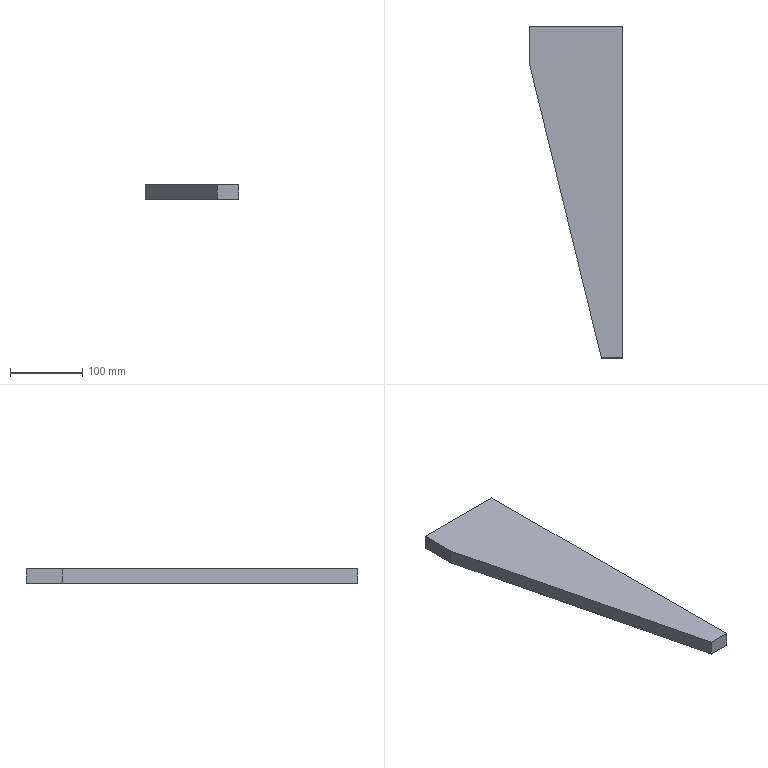Part | SolidWorks | features Cut 1, Extrusion 1 | 1 solid | 7 faces | box 130 x 460 x 20 mm | volume 786000 mm3 | plane 7
STEP:
#1=CARTESIAN_POINT('',(-65.,230.,-10.));
#2=VERTEX_POINT('',#1);
#3=CARTESIAN_POINT('',(-65.,180.,-10.));
#4=VERTEX_POINT('',#3);
#5=CARTESIAN_POINT('',(-65.,-230.,-10.));
#6=DIRECTION('',(0.,-1.,0.));
#7=VECTOR('',#6,1000.);
#8=LINE('',#5,#7);
#9=EDGE_CURVE('',#2,#4,#8,.T.);
#10=ORIENTED_EDGE('',*,*,#9,.T.);
#11=CARTESIAN_POINT('',(-65.,180.,10.));
#12=VERTEX_POINT('',#11);
#13=CARTESIAN_POINT('',(-65.,180.,-10.));
#14=DIRECTION('',(0.,0.,1.));
#15=VECTOR('',#14,1000.);
#16=LINE('',#13,#15);
#17=EDGE_CURVE('',#4,#12,#16,.T.);
#18=ORIENTED_EDGE('',*,*,#17,.T.);
#19=CARTESIAN_POINT('',(-65.,230.,10.));
#20=VERTEX_POINT('',#19);
#21=CARTESIAN_POINT('',(-65.,-230.,10.));
#22=DIRECTION('',(0.,-1.,0.));
#23=VECTOR('',#22,1000.);
#24=LINE('',#21,#23);
#25=EDGE_CURVE('',#20,#12,#24,.T.);
#26=ORIENTED_EDGE('',*,*,#25,.F.);
#27=CARTESIAN_POINT('',(-65.,230.,10.));
#28=DIRECTION('',(0.,0.,-1.));
#29=VECTOR('',#28,1000.);
#30=LINE('',#27,#29);
#31=EDGE_CURVE('',#20,#2,#30,.T.);
#32=ORIENTED_EDGE('',*,*,#31,.T.);
#33=EDGE_LOOP('',(#10,#18,#26,#32));
#34=FACE_OUTER_BOUND('',#33,.T.);
#35=CARTESIAN_POINT('',(-65.,-230.,10.));
#36=DIRECTION('',(1.,0.,0.));
#37=DIRECTION('',(0.,0.,-1.));
#38=AXIS2_PLACEMENT_3D('',#35,#36,#37);
#39=PLANE('',#38);
#40=ADVANCED_FACE('',(#34),#39,.F.);
#41=CARTESIAN_POINT('',(35.,-230.,10.));
#42=VERTEX_POINT('',#41);
#43=CARTESIAN_POINT('',(65.,-230.,10.));
#44=VERTEX_POINT('',#43);
#45=CARTESIAN_POINT('',(65.,-230.,10.));
#46=DIRECTION('',(1.,0.,0.));
#47=VECTOR('',#46,1000.);
#48=LINE('',#45,#47);
#49=EDGE_CURVE('',#42,#44,#48,.T.);
#50=ORIENTED_EDGE('',*,*,#49,.F.);
#51=CARTESIAN_POINT('',(35.,-230.,-10.));
#52=VERTEX_POINT('',#51);
#53=CARTESIAN_POINT('',(35.,-230.,-10.));
#54=DIRECTION('',(0.,0.,1.));
#55=VECTOR('',#54,1000.);
#56=LINE('',#53,#55);
#57=EDGE_CURVE('',#52,#42,#56,.T.);
#58=ORIENTED_EDGE('',*,*,#57,.F.);
#59=CARTESIAN_POINT('',(65.,-230.,-10.));
#60=VERTEX_POINT('',#59);
#61=CARTESIAN_POINT('',(65.,-230.,-10.));
#62=DIRECTION('',(1.,0.,0.));
#63=VECTOR('',#62,1000.);
#64=LINE('',#61,#63);
#65=EDGE_CURVE('',#52,#60,#64,.T.);
#66=ORIENTED_EDGE('',*,*,#65,.T.);
#67=CARTESIAN_POINT('',(65.,-230.,10.));
#68=DIRECTION('',(0.,0.,-1.));
#69=VECTOR('',#68,1000.);
#70=LINE('',#67,#69);
#71=EDGE_CURVE('',#44,#60,#70,.T.);
#72=ORIENTED_EDGE('',*,*,#71,.F.);
#73=EDGE_LOOP('',(#50,#58,#66,#72));
#74=FACE_OUTER_BOUND('',#73,.T.);
#75=CARTESIAN_POINT('',(65.,-230.,10.));
#76=DIRECTION('',(0.,1.,0.));
#77=DIRECTION('',(0.,0.,1.));
#78=AXIS2_PLACEMENT_3D('',#75,#76,#77);
#79=PLANE('',#78);
#80=ADVANCED_FACE('',(#74),#79,.F.);
#81=CARTESIAN_POINT('',(65.,230.,-10.));
#82=VERTEX_POINT('',#81);
#83=CARTESIAN_POINT('',(65.,-230.,-10.));
#84=DIRECTION('',(0.,1.,0.));
#85=VECTOR('',#84,1000.);
#86=LINE('',#83,#85);
#87=EDGE_CURVE('',#60,#82,#86,.T.);
#88=ORIENTED_EDGE('',*,*,#87,.T.);
#89=CARTESIAN_POINT('',(65.,230.,10.));
#90=VERTEX_POINT('',#89);
#91=CARTESIAN_POINT('',(65.,230.,10.));
#92=DIRECTION('',(0.,0.,-1.));
#93=VECTOR('',#92,1000.);
#94=LINE('',#91,#93);
#95=EDGE_CURVE('',#90,#82,#94,.T.);
#96=ORIENTED_EDGE('',*,*,#95,.F.);
#97=CARTESIAN_POINT('',(65.,-230.,10.));
#98=DIRECTION('',(0.,1.,0.));
#99=VECTOR('',#98,1000.);
#100=LINE('',#97,#99);
#101=EDGE_CURVE('',#44,#90,#100,.T.);
#102=ORIENTED_EDGE('',*,*,#101,.F.);
#103=ORIENTED_EDGE('',*,*,#71,.T.);
#104=EDGE_LOOP('',(#88,#96,#102,#103));
#105=FACE_OUTER_BOUND('',#104,.T.);
#106=CARTESIAN_POINT('',(65.,-230.,10.));
#107=DIRECTION('',(-1.,0.,0.));
#108=DIRECTION('',(0.,0.,1.));
#109=AXIS2_PLACEMENT_3D('',#106,#107,#108);
#110=PLANE('',#109);
#111=ADVANCED_FACE('',(#105),#110,.F.);
#112=CARTESIAN_POINT('',(65.,230.,-10.));
#113=DIRECTION('',(-1.,0.,0.));
#114=VECTOR('',#113,1000.);
#115=LINE('',#112,#114);
#116=EDGE_CURVE('',#82,#2,#115,.T.);
#117=ORIENTED_EDGE('',*,*,#116,.T.);
#118=ORIENTED_EDGE('',*,*,#31,.F.);
#119=CARTESIAN_POINT('',(65.,230.,10.));
#120=DIRECTION('',(-1.,0.,0.));
#121=VECTOR('',#120,1000.);
#122=LINE('',#119,#121);
#123=EDGE_CURVE('',#90,#20,#122,.T.);
#124=ORIENTED_EDGE('',*,*,#123,.F.);
#125=ORIENTED_EDGE('',*,*,#95,.T.);
#126=EDGE_LOOP('',(#117,#118,#124,#125));
#127=FACE_OUTER_BOUND('',#126,.T.);
#128=CARTESIAN_POINT('',(65.,230.,10.));
#129=DIRECTION('',(0.,-1.,0.));
#130=DIRECTION('',(0.,0.,-1.));
#131=AXIS2_PLACEMENT_3D('',#128,#129,#130);
#132=PLANE('',#131);
#133=ADVANCED_FACE('',(#127),#132,.F.);
#134=CARTESIAN_POINT('',(-65.,180.,10.));
#135=DIRECTION('',(-0.237,0.9715,0.));
#136=VECTOR('',#135,1000.);
#137=LINE('',#134,#136);
#138=EDGE_CURVE('',#42,#12,#137,.T.);
#139=ORIENTED_EDGE('',*,*,#138,.F.);
#140=ORIENTED_EDGE('',*,*,#49,.T.);
#141=ORIENTED_EDGE('',*,*,#101,.T.);
#142=ORIENTED_EDGE('',*,*,#123,.T.);
#143=ORIENTED_EDGE('',*,*,#25,.T.);
#144=EDGE_LOOP('',(#139,#140,#141,#142,#143));
#145=FACE_OUTER_BOUND('',#144,.T.);
#146=CARTESIAN_POINT('',(0.,0.,10.));
#147=DIRECTION('',(0.,0.,1.));
#148=DIRECTION('',(1.,0.,0.));
#149=AXIS2_PLACEMENT_3D('',#146,#147,#148);
#150=PLANE('',#149);
#151=ADVANCED_FACE('',(#145),#150,.T.);
#152=ORIENTED_EDGE('',*,*,#65,.F.);
#153=CARTESIAN_POINT('',(-65.,180.,-10.));
#154=DIRECTION('',(-0.237,0.9715,0.));
#155=VECTOR('',#154,1000.);
#156=LINE('',#153,#155);
#157=EDGE_CURVE('',#52,#4,#156,.T.);
#158=ORIENTED_EDGE('',*,*,#157,.T.);
#159=ORIENTED_EDGE('',*,*,#9,.F.);
#160=ORIENTED_EDGE('',*,*,#116,.F.);
#161=ORIENTED_EDGE('',*,*,#87,.F.);
#162=EDGE_LOOP('',(#152,#158,#159,#160,#161));
#163=FACE_OUTER_BOUND('',#162,.T.);
#164=CARTESIAN_POINT('',(0.,0.,-10.));
#165=DIRECTION('',(0.,0.,1.));
#166=DIRECTION('',(1.,0.,0.));
#167=AXIS2_PLACEMENT_3D('',#164,#165,#166);
#168=PLANE('',#167);
#169=ADVANCED_FACE('',(#163),#168,.F.);
#170=ORIENTED_EDGE('',*,*,#138,.T.);
#171=ORIENTED_EDGE('',*,*,#17,.F.);
#172=ORIENTED_EDGE('',*,*,#157,.F.);
#173=ORIENTED_EDGE('',*,*,#57,.T.);
#174=EDGE_LOOP('',(#170,#171,#172,#173));
#175=FACE_OUTER_BOUND('',#174,.T.);
#176=CARTESIAN_POINT('',(-65.,180.,-10.));
#177=DIRECTION('',(0.9715,0.237,0.));
#178=DIRECTION('',(-0.237,0.9715,0.));
#179=AXIS2_PLACEMENT_3D('',#176,#177,#178);
#180=PLANE('',#179);
#181=ADVANCED_FACE('',(#175),#180,.F.);
#182=CLOSED_SHELL('',(#40,#80,#111,#133,#151,#169,#181));
#183=MANIFOLD_SOLID_BREP('',#182);
#184=CARTESIAN_POINT('',(0.,0.,0.));
#185=DIRECTION('',(0.,0.,1.));
#186=DIRECTION('',(1.,0.,0.));
#187=AXIS2_PLACEMENT_3D('',#184,#185,#186);
#188=(LENGTH_UNIT()NAMED_UNIT(*)SI_UNIT(.MILLI.,.METRE.));
#189=UNCERTAINTY_MEASURE_WITH_UNIT(LENGTH_MEASURE(0.00001),#188,'','');
#190=(NAMED_UNIT(*)PLANE_ANGLE_UNIT()SI_UNIT($,.RADIAN.));
#191=(NAMED_UNIT(*)SI_UNIT($,.STERADIAN.)SOLID_ANGLE_UNIT());
#192=(GEOMETRIC_REPRESENTATION_CONTEXT(3)GLOBAL_UNCERTAINTY_ASSIGNED_CONTEXT((#189))GLOBAL_UNIT_ASSIGNED_CONTEXT((#188,#190,#191))REPRESENTATION_CONTEXT('',''));
#193=ADVANCED_BREP_SHAPE_REPRESENTATION('',(#183,#187),#192);